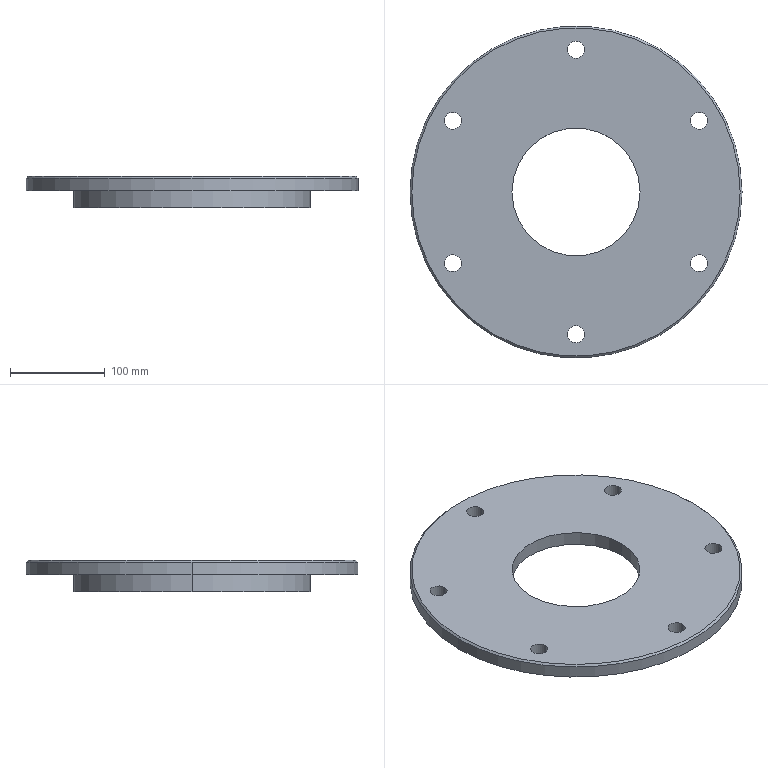Part | SolidWorks | features ICE 2, Chamfer 1, Extrusion 1 | 1 solid | 26 faces | box 350 x 350 x 33 mm | volume 1402702 mm3 | cylinder 20 | plane 4 | cone 2 | commonest cylinder face diameters 18 x12 135 x2 220 x2 250 x2 350 x2
STEP:
#1=CARTESIAN_POINT('',(-67.5,0.,18.));
#2=VERTEX_POINT('',#1);
#3=CARTESIAN_POINT('',(67.5,0.,18.));
#4=VERTEX_POINT('',#3);
#5=CARTESIAN_POINT('',(0.,0.,18.));
#6=DIRECTION('',(0.,0.,1.));
#7=DIRECTION('',(1.,0.,0.));
#8=AXIS2_PLACEMENT_3D('',#5,#6,#7);
#9=CIRCLE('',#8,67.5);
#10=EDGE_CURVE('',#2,#4,#9,.T.);
#11=ORIENTED_EDGE('',*,*,#10,.F.);
#12=CARTESIAN_POINT('',(-67.5,0.,33.));
#13=VERTEX_POINT('',#12);
#14=CARTESIAN_POINT('',(-67.5,0.,0.));
#15=DIRECTION('',(0.,0.,1.));
#16=VECTOR('',#15,1000.);
#17=LINE('',#14,#16);
#18=EDGE_CURVE('',#2,#13,#17,.T.);
#19=ORIENTED_EDGE('',*,*,#18,.T.);
#20=CARTESIAN_POINT('',(67.5,0.,33.));
#21=VERTEX_POINT('',#20);
#22=CARTESIAN_POINT('',(0.,0.,33.));
#23=DIRECTION('',(0.,0.,1.));
#24=DIRECTION('',(1.,0.,0.));
#25=AXIS2_PLACEMENT_3D('',#22,#23,#24);
#26=CIRCLE('',#25,67.5);
#27=EDGE_CURVE('',#13,#21,#26,.T.);
#28=ORIENTED_EDGE('',*,*,#27,.T.);
#29=CARTESIAN_POINT('',(67.5,0.,0.));
#30=DIRECTION('',(0.,0.,1.));
#31=VECTOR('',#30,1000.);
#32=LINE('',#29,#31);
#33=EDGE_CURVE('',#4,#21,#32,.T.);
#34=ORIENTED_EDGE('',*,*,#33,.F.);
#35=EDGE_LOOP('',(#11,#19,#28,#34));
#36=FACE_OUTER_BOUND('',#35,.T.);
#37=CARTESIAN_POINT('',(0.,0.,0.));
#38=DIRECTION('',(0.,0.,1.));
#39=DIRECTION('',(1.,0.,0.));
#40=AXIS2_PLACEMENT_3D('',#37,#38,#39);
#41=CYLINDRICAL_SURFACE('',#40,67.5);
#42=ADVANCED_FACE('',(#36),#41,.F.);
#43=CARTESIAN_POINT('',(173.,0.,33.));
#44=VERTEX_POINT('',#43);
#45=CARTESIAN_POINT('',(-173.,0.,33.));
#46=VERTEX_POINT('',#45);
#47=CARTESIAN_POINT('',(0.,0.,33.));
#48=DIRECTION('',(0.,0.,1.));
#49=DIRECTION('',(1.,0.,0.));
#50=AXIS2_PLACEMENT_3D('',#47,#48,#49);
#51=CIRCLE('',#50,173.);
#52=EDGE_CURVE('',#44,#46,#51,.T.);
#53=ORIENTED_EDGE('',*,*,#52,.F.);
#54=CARTESIAN_POINT('',(175.,0.,31.));
#55=VERTEX_POINT('',#54);
#56=CARTESIAN_POINT('',(173.,0.,33.));
#57=DIRECTION('',(0.7071,0.,-0.7071));
#58=VECTOR('',#57,1000.);
#59=LINE('',#56,#58);
#60=EDGE_CURVE('',#44,#55,#59,.T.);
#61=ORIENTED_EDGE('',*,*,#60,.T.);
#62=CARTESIAN_POINT('',(-175.,0.,31.));
#63=VERTEX_POINT('',#62);
#64=CARTESIAN_POINT('',(0.,0.,31.));
#65=DIRECTION('',(0.,0.,-1.));
#66=DIRECTION('',(1.,0.,0.));
#67=AXIS2_PLACEMENT_3D('',#64,#65,#66);
#68=CIRCLE('',#67,175.);
#69=EDGE_CURVE('',#63,#55,#68,.T.);
#70=ORIENTED_EDGE('',*,*,#69,.F.);
#71=CARTESIAN_POINT('',(-173.,0.,33.));
#72=DIRECTION('',(-0.7071,0.,-0.7071));
#73=VECTOR('',#72,1000.);
#74=LINE('',#71,#73);
#75=EDGE_CURVE('',#46,#63,#74,.T.);
#76=ORIENTED_EDGE('',*,*,#75,.F.);
#77=EDGE_LOOP('',(#53,#61,#70,#76));
#78=FACE_OUTER_BOUND('',#77,.T.);
#79=CARTESIAN_POINT('',(0.,0.,33.));
#80=DIRECTION('',(0.,0.,-1.));
#81=DIRECTION('',(-1.,0.,0.));
#82=AXIS2_PLACEMENT_3D('',#79,#80,#81);
#83=CONICAL_SURFACE('',#82,173.,0.7854);
#84=ADVANCED_FACE('',(#78),#83,.T.);
#85=CARTESIAN_POINT('',(120.904,75.,33.));
#86=VERTEX_POINT('',#85);
#87=CARTESIAN_POINT('',(138.904,75.,33.));
#88=VERTEX_POINT('',#87);
#89=CARTESIAN_POINT('',(129.904,75.,33.));
#90=DIRECTION('',(0.,0.,1.));
#91=DIRECTION('',(1.,0.,0.));
#92=AXIS2_PLACEMENT_3D('',#89,#90,#91);
#93=CIRCLE('',#92,9.);
#94=EDGE_CURVE('',#86,#88,#93,.T.);
#95=ORIENTED_EDGE('',*,*,#94,.T.);
#96=CARTESIAN_POINT('',(138.904,75.,18.));
#97=VERTEX_POINT('',#96);
#98=CARTESIAN_POINT('',(138.904,75.,33.));
#99=DIRECTION('',(0.,0.,-1.));
#100=VECTOR('',#99,1000.);
#101=LINE('',#98,#100);
#102=EDGE_CURVE('',#88,#97,#101,.T.);
#103=ORIENTED_EDGE('',*,*,#102,.T.);
#104=CARTESIAN_POINT('',(120.904,75.,18.));
#105=VERTEX_POINT('',#104);
#106=CARTESIAN_POINT('',(129.904,75.,18.));
#107=DIRECTION('',(0.,0.,1.));
#108=DIRECTION('',(1.,0.,0.));
#109=AXIS2_PLACEMENT_3D('',#106,#107,#108);
#110=CIRCLE('',#109,9.);
#111=EDGE_CURVE('',#105,#97,#110,.T.);
#112=ORIENTED_EDGE('',*,*,#111,.F.);
#113=CARTESIAN_POINT('',(120.904,75.,33.));
#114=DIRECTION('',(0.,0.,-1.));
#115=VECTOR('',#114,1000.);
#116=LINE('',#113,#115);
#117=EDGE_CURVE('',#86,#105,#116,.T.);
#118=ORIENTED_EDGE('',*,*,#117,.F.);
#119=EDGE_LOOP('',(#95,#103,#112,#118));
#120=FACE_OUTER_BOUND('',#119,.T.);
#121=CARTESIAN_POINT('',(129.904,75.,33.));
#122=DIRECTION('',(0.,0.,-1.));
#123=DIRECTION('',(-1.,0.,0.));
#124=AXIS2_PLACEMENT_3D('',#121,#122,#123);
#125=CYLINDRICAL_SURFACE('',#124,9.);
#126=ADVANCED_FACE('',(#120),#125,.F.);
#127=CARTESIAN_POINT('',(120.904,-75.,33.));
#128=VERTEX_POINT('',#127);
#129=CARTESIAN_POINT('',(138.904,-75.,33.));
#130=VERTEX_POINT('',#129);
#131=CARTESIAN_POINT('',(129.904,-75.,33.));
#132=DIRECTION('',(0.,0.,1.));
#133=DIRECTION('',(1.,0.,0.));
#134=AXIS2_PLACEMENT_3D('',#131,#132,#133);
#135=CIRCLE('',#134,9.);
#136=EDGE_CURVE('',#128,#130,#135,.T.);
#137=ORIENTED_EDGE('',*,*,#136,.T.);
#138=CARTESIAN_POINT('',(138.904,-75.,18.));
#139=VERTEX_POINT('',#138);
#140=CARTESIAN_POINT('',(138.904,-75.,33.));
#141=DIRECTION('',(0.,0.,-1.));
#142=VECTOR('',#141,1000.);
#143=LINE('',#140,#142);
#144=EDGE_CURVE('',#130,#139,#143,.T.);
#145=ORIENTED_EDGE('',*,*,#144,.T.);
#146=CARTESIAN_POINT('',(120.904,-75.,18.));
#147=VERTEX_POINT('',#146);
#148=CARTESIAN_POINT('',(129.904,-75.,18.));
#149=DIRECTION('',(0.,0.,1.));
#150=DIRECTION('',(1.,0.,0.));
#151=AXIS2_PLACEMENT_3D('',#148,#149,#150);
#152=CIRCLE('',#151,9.);
#153=EDGE_CURVE('',#147,#139,#152,.T.);
#154=ORIENTED_EDGE('',*,*,#153,.F.);
#155=CARTESIAN_POINT('',(120.904,-75.,33.));
#156=DIRECTION('',(0.,0.,-1.));
#157=VECTOR('',#156,1000.);
#158=LINE('',#155,#157);
#159=EDGE_CURVE('',#128,#147,#158,.T.);
#160=ORIENTED_EDGE('',*,*,#159,.F.);
#161=EDGE_LOOP('',(#137,#145,#154,#160));
#162=FACE_OUTER_BOUND('',#161,.T.);
#163=CARTESIAN_POINT('',(129.904,-75.,33.));
#164=DIRECTION('',(0.,0.,-1.));
#165=DIRECTION('',(-1.,0.,0.));
#166=AXIS2_PLACEMENT_3D('',#163,#164,#165);
#167=CYLINDRICAL_SURFACE('',#166,9.);
#168=ADVANCED_FACE('',(#162),#167,.F.);
#169=CARTESIAN_POINT('',(-9.,-150.,33.));
#170=VERTEX_POINT('',#169);
#171=CARTESIAN_POINT('',(9.,-150.,33.));
#172=VERTEX_POINT('',#171);
#173=CARTESIAN_POINT('',(0.,-150.,33.));
#174=DIRECTION('',(0.,0.,1.));
#175=DIRECTION('',(1.,0.,0.));
#176=AXIS2_PLACEMENT_3D('',#173,#174,#175);
#177=CIRCLE('',#176,9.);
#178=EDGE_CURVE('',#170,#172,#177,.T.);
#179=ORIENTED_EDGE('',*,*,#178,.T.);
#180=CARTESIAN_POINT('',(9.,-150.,18.));
#181=VERTEX_POINT('',#180);
#182=CARTESIAN_POINT('',(9.,-150.,33.));
#183=DIRECTION('',(0.,0.,-1.));
#184=VECTOR('',#183,1000.);
#185=LINE('',#182,#184);
#186=EDGE_CURVE('',#172,#181,#185,.T.);
#187=ORIENTED_EDGE('',*,*,#186,.T.);
#188=CARTESIAN_POINT('',(-9.,-150.,18.));
#189=VERTEX_POINT('',#188);
#190=CARTESIAN_POINT('',(0.,-150.,18.));
#191=DIRECTION('',(0.,0.,1.));
#192=DIRECTION('',(1.,0.,0.));
#193=AXIS2_PLACEMENT_3D('',#190,#191,#192);
#194=CIRCLE('',#193,9.);
#195=EDGE_CURVE('',#189,#181,#194,.T.);
#196=ORIENTED_EDGE('',*,*,#195,.F.);
#197=CARTESIAN_POINT('',(-9.,-150.,33.));
#198=DIRECTION('',(0.,0.,-1.));
#199=VECTOR('',#198,1000.);
#200=LINE('',#197,#199);
#201=EDGE_CURVE('',#170,#189,#200,.T.);
#202=ORIENTED_EDGE('',*,*,#201,.F.);
#203=EDGE_LOOP('',(#179,#187,#196,#202));
#204=FACE_OUTER_BOUND('',#203,.T.);
#205=CARTESIAN_POINT('',(0.,-150.,33.));
#206=DIRECTION('',(0.,0.,-1.));
#207=DIRECTION('',(-1.,0.,0.));
#208=AXIS2_PLACEMENT_3D('',#205,#206,#207);
#209=CYLINDRICAL_SURFACE('',#208,9.);
#210=ADVANCED_FACE('',(#204),#209,.F.);
#211=CARTESIAN_POINT('',(-138.904,-75.,33.));
#212=VERTEX_POINT('',#211);
#213=CARTESIAN_POINT('',(-120.904,-75.,33.));
#214=VERTEX_POINT('',#213);
#215=CARTESIAN_POINT('',(-129.904,-75.,33.));
#216=DIRECTION('',(0.,0.,1.));
#217=DIRECTION('',(1.,0.,0.));
#218=AXIS2_PLACEMENT_3D('',#215,#216,#217);
#219=CIRCLE('',#218,9.);
#220=EDGE_CURVE('',#212,#214,#219,.T.);
#221=ORIENTED_EDGE('',*,*,#220,.T.);
#222=CARTESIAN_POINT('',(-120.904,-75.,18.));
#223=VERTEX_POINT('',#222);
#224=CARTESIAN_POINT('',(-120.904,-75.,33.));
#225=DIRECTION('',(0.,0.,-1.));
#226=VECTOR('',#225,1000.);
#227=LINE('',#224,#226);
#228=EDGE_CURVE('',#214,#223,#227,.T.);
#229=ORIENTED_EDGE('',*,*,#228,.T.);
#230=CARTESIAN_POINT('',(-138.904,-75.,18.));
#231=VERTEX_POINT('',#230);
#232=CARTESIAN_POINT('',(-129.904,-75.,18.));
#233=DIRECTION('',(0.,0.,1.));
#234=DIRECTION('',(1.,0.,0.));
#235=AXIS2_PLACEMENT_3D('',#232,#233,#234);
#236=CIRCLE('',#235,9.);
#237=EDGE_CURVE('',#231,#223,#236,.T.);
#238=ORIENTED_EDGE('',*,*,#237,.F.);
#239=CARTESIAN_POINT('',(-138.904,-75.,33.));
#240=DIRECTION('',(0.,0.,-1.));
#241=VECTOR('',#240,1000.);
#242=LINE('',#239,#241);
#243=EDGE_CURVE('',#212,#231,#242,.T.);
#244=ORIENTED_EDGE('',*,*,#243,.F.);
#245=EDGE_LOOP('',(#221,#229,#238,#244));
#246=FACE_OUTER_BOUND('',#245,.T.);
#247=CARTESIAN_POINT('',(-129.904,-75.,33.));
#248=DIRECTION('',(0.,0.,-1.));
#249=DIRECTION('',(-1.,0.,0.));
#250=AXIS2_PLACEMENT_3D('',#247,#248,#249);
#251=CYLINDRICAL_SURFACE('',#250,9.);
#252=ADVANCED_FACE('',(#246),#251,.F.);
#253=CARTESIAN_POINT('',(-138.904,75.,33.));
#254=VERTEX_POINT('',#253);
#255=CARTESIAN_POINT('',(-120.904,75.,33.));
#256=VERTEX_POINT('',#255);
#257=CARTESIAN_POINT('',(-129.904,75.,33.));
#258=DIRECTION('',(0.,0.,1.));
#259=DIRECTION('',(1.,0.,0.));
#260=AXIS2_PLACEMENT_3D('',#257,#258,#259);
#261=CIRCLE('',#260,9.);
#262=EDGE_CURVE('',#254,#256,#261,.T.);
#263=ORIENTED_EDGE('',*,*,#262,.T.);
#264=CARTESIAN_POINT('',(-120.904,75.,18.));
#265=VERTEX_POINT('',#264);
#266=CARTESIAN_POINT('',(-120.904,75.,33.));
#267=DIRECTION('',(0.,0.,-1.));
#268=VECTOR('',#267,1000.);
#269=LINE('',#266,#268);
#270=EDGE_CURVE('',#256,#265,#269,.T.);
#271=ORIENTED_EDGE('',*,*,#270,.T.);
#272=CARTESIAN_POINT('',(-138.904,75.,18.));
#273=VERTEX_POINT('',#272);
#274=CARTESIAN_POINT('',(-129.904,75.,18.));
#275=DIRECTION('',(0.,0.,1.));
#276=DIRECTION('',(1.,0.,0.));
#277=AXIS2_PLACEMENT_3D('',#274,#275,#276);
#278=CIRCLE('',#277,9.);
#279=EDGE_CURVE('',#273,#265,#278,.T.);
#280=ORIENTED_EDGE('',*,*,#279,.F.);
#281=CARTESIAN_POINT('',(-138.904,75.,33.));
#282=DIRECTION('',(0.,0.,-1.));
#283=VECTOR('',#282,1000.);
#284=LINE('',#281,#283);
#285=EDGE_CURVE('',#254,#273,#284,.T.);
#286=ORIENTED_EDGE('',*,*,#285,.F.);
#287=EDGE_LOOP('',(#263,#271,#280,#286));
#288=FACE_OUTER_BOUND('',#287,.T.);
#289=CARTESIAN_POINT('',(-129.904,75.,33.));
#290=DIRECTION('',(0.,0.,-1.));
#291=DIRECTION('',(-1.,0.,0.));
#292=AXIS2_PLACEMENT_3D('',#289,#290,#291);
#293=CYLINDRICAL_SURFACE('',#292,9.);
#294=ADVANCED_FACE('',(#288),#293,.F.);
#295=CARTESIAN_POINT('',(-9.,150.,33.));
#296=VERTEX_POINT('',#295);
#297=CARTESIAN_POINT('',(9.,150.,33.));
#298=VERTEX_POINT('',#297);
#299=CARTESIAN_POINT('',(0.,150.,33.));
#300=DIRECTION('',(0.,0.,1.));
#301=DIRECTION('',(1.,0.,0.));
#302=AXIS2_PLACEMENT_3D('',#299,#300,#301);
#303=CIRCLE('',#302,9.);
#304=EDGE_CURVE('',#296,#298,#303,.T.);
#305=ORIENTED_EDGE('',*,*,#304,.T.);
#306=CARTESIAN_POINT('',(9.,150.,18.));
#307=VERTEX_POINT('',#306);
#308=CARTESIAN_POINT('',(9.,150.,33.));
#309=DIRECTION('',(0.,0.,-1.));
#310=VECTOR('',#309,1000.);
#311=LINE('',#308,#310);
#312=EDGE_CURVE('',#298,#307,#311,.T.);
#313=ORIENTED_EDGE('',*,*,#312,.T.);
#314=CARTESIAN_POINT('',(-9.,150.,18.));
#315=VERTEX_POINT('',#314);
#316=CARTESIAN_POINT('',(0.,150.,18.));
#317=DIRECTION('',(0.,0.,1.));
#318=DIRECTION('',(1.,0.,0.));
#319=AXIS2_PLACEMENT_3D('',#316,#317,#318);
#320=CIRCLE('',#319,9.);
#321=EDGE_CURVE('',#315,#307,#320,.T.);
#322=ORIENTED_EDGE('',*,*,#321,.F.);
#323=CARTESIAN_POINT('',(-9.,150.,33.));
#324=DIRECTION('',(0.,0.,-1.));
#325=VECTOR('',#324,1000.);
#326=LINE('',#323,#325);
#327=EDGE_CURVE('',#296,#315,#326,.T.);
#328=ORIENTED_EDGE('',*,*,#327,.F.);
#329=EDGE_LOOP('',(#305,#313,#322,#328));
#330=FACE_OUTER_BOUND('',#329,.T.);
#331=CARTESIAN_POINT('',(0.,150.,33.));
#332=DIRECTION('',(0.,0.,-1.));
#333=DIRECTION('',(-1.,0.,0.));
#334=AXIS2_PLACEMENT_3D('',#331,#332,#333);
#335=CYLINDRICAL_SURFACE('',#334,9.);
#336=ADVANCED_FACE('',(#330),#335,.F.);
#337=ORIENTED_EDGE('',*,*,#69,.T.);
#338=CARTESIAN_POINT('',(175.,0.,18.));
#339=VERTEX_POINT('',#338);
#340=CARTESIAN_POINT('',(175.,0.,33.));
#341=DIRECTION('',(0.,0.,-1.));
#342=VECTOR('',#341,1000.);
#343=LINE('',#340,#342);
#344=EDGE_CURVE('',#55,#339,#343,.T.);
#345=ORIENTED_EDGE('',*,*,#344,.T.);
#346=CARTESIAN_POINT('',(-175.,0.,18.));
#347=VERTEX_POINT('',#346);
#348=CARTESIAN_POINT('',(0.,0.,18.));
#349=DIRECTION('',(0.,0.,1.));
#350=DIRECTION('',(1.,0.,0.));
#351=AXIS2_PLACEMENT_3D('',#348,#349,#350);
#352=CIRCLE('',#351,175.);
#353=EDGE_CURVE('',#339,#347,#352,.T.);
#354=ORIENTED_EDGE('',*,*,#353,.T.);
#355=CARTESIAN_POINT('',(-175.,0.,33.));
#356=DIRECTION('',(0.,0.,-1.));
#357=VECTOR('',#356,1000.);
#358=LINE('',#355,#357);
#359=EDGE_CURVE('',#63,#347,#358,.T.);
#360=ORIENTED_EDGE('',*,*,#359,.F.);
#361=EDGE_LOOP('',(#337,#345,#354,#360));
#362=FACE_OUTER_BOUND('',#361,.T.);
#363=CARTESIAN_POINT('',(0.,0.,33.));
#364=DIRECTION('',(0.,0.,-1.));
#365=DIRECTION('',(-1.,0.,0.));
#366=AXIS2_PLACEMENT_3D('',#363,#364,#365);
#367=CYLINDRICAL_SURFACE('',#366,175.);
#368=ADVANCED_FACE('',(#362),#367,.T.);
#369=CARTESIAN_POINT('',(110.,0.,18.));
#370=VERTEX_POINT('',#369);
#371=CARTESIAN_POINT('',(-110.,0.,18.));
#372=VERTEX_POINT('',#371);
#373=CARTESIAN_POINT('',(0.,0.,18.));
#374=DIRECTION('',(0.,0.,-1.));
#375=DIRECTION('',(-1.,0.,0.));
#376=AXIS2_PLACEMENT_3D('',#373,#374,#375);
#377=CIRCLE('',#376,110.);
#378=EDGE_CURVE('',#370,#372,#377,.T.);
#379=ORIENTED_EDGE('',*,*,#378,.F.);
#380=CARTESIAN_POINT('',(110.,0.,0.));
#381=VERTEX_POINT('',#380);
#382=CARTESIAN_POINT('',(110.,0.,371.553));
#383=DIRECTION('',(0.,0.,-1.));
#384=VECTOR('',#383,1000.);
#385=LINE('',#382,#384);
#386=EDGE_CURVE('',#370,#381,#385,.T.);
#387=ORIENTED_EDGE('',*,*,#386,.T.);
#388=CARTESIAN_POINT('',(-110.,0.,0.));
#389=VERTEX_POINT('',#388);
#390=CARTESIAN_POINT('',(0.,0.,0.));
#391=DIRECTION('',(0.,0.,1.));
#392=DIRECTION('',(1.,0.,0.));
#393=AXIS2_PLACEMENT_3D('',#390,#391,#392);
#394=CIRCLE('',#393,110.);
#395=EDGE_CURVE('',#389,#381,#394,.T.);
#396=ORIENTED_EDGE('',*,*,#395,.F.);
#397=CARTESIAN_POINT('',(-110.,0.,371.553));
#398=DIRECTION('',(0.,0.,-1.));
#399=VECTOR('',#398,1000.);
#400=LINE('',#397,#399);
#401=EDGE_CURVE('',#372,#389,#400,.T.);
#402=ORIENTED_EDGE('',*,*,#401,.F.);
#403=EDGE_LOOP('',(#379,#387,#396,#402));
#404=FACE_OUTER_BOUND('',#403,.T.);
#405=CARTESIAN_POINT('',(0.,0.,371.553));
#406=DIRECTION('',(0.,0.,-1.));
#407=DIRECTION('',(-1.,0.,0.));
#408=AXIS2_PLACEMENT_3D('',#405,#406,#407);
#409=CYLINDRICAL_SURFACE('',#408,110.);
#410=ADVANCED_FACE('',(#404),#409,.F.);
#411=CARTESIAN_POINT('',(125.,0.,18.));
#412=VERTEX_POINT('',#411);
#413=CARTESIAN_POINT('',(-125.,0.,18.));
#414=VERTEX_POINT('',#413);
#415=CARTESIAN_POINT('',(0.,0.,18.));
#416=DIRECTION('',(0.,0.,1.));
#417=DIRECTION('',(1.,0.,0.));
#418=AXIS2_PLACEMENT_3D('',#415,#416,#417);
#419=CIRCLE('',#418,125.);
#420=EDGE_CURVE('',#412,#414,#419,.T.);
#421=ORIENTED_EDGE('',*,*,#420,.F.);
#422=CARTESIAN_POINT('',(125.,0.,0.));
#423=VERTEX_POINT('',#422);
#424=CARTESIAN_POINT('',(125.,0.,371.553));
#425=DIRECTION('',(0.,0.,-1.));
#426=VECTOR('',#425,1000.);
#427=LINE('',#424,#426);
#428=EDGE_CURVE('',#412,#423,#427,.T.);
#429=ORIENTED_EDGE('',*,*,#428,.T.);
#430=CARTESIAN_POINT('',(-125.,0.,0.));
#431=VERTEX_POINT('',#430);
#432=CARTESIAN_POINT('',(0.,0.,0.));
#433=DIRECTION('',(0.,0.,1.));
#434=DIRECTION('',(1.,0.,0.));
#435=AXIS2_PLACEMENT_3D('',#432,#433,#434);
#436=CIRCLE('',#435,125.);
#437=EDGE_CURVE('',#423,#431,#436,.T.);
#438=ORIENTED_EDGE('',*,*,#437,.T.);
#439=CARTESIAN_POINT('',(-125.,0.,371.553));
#440=DIRECTION('',(0.,0.,-1.));
#441=VECTOR('',#440,1000.);
#442=LINE('',#439,#441);
#443=EDGE_CURVE('',#414,#431,#442,.T.);
#444=ORIENTED_EDGE('',*,*,#443,.F.);
#445=EDGE_LOOP('',(#421,#429,#438,#444));
#446=FACE_OUTER_BOUND('',#445,.T.);
#447=CARTESIAN_POINT('',(0.,0.,371.553));
#448=DIRECTION('',(0.,0.,-1.));
#449=DIRECTION('',(-1.,0.,0.));
#450=AXIS2_PLACEMENT_3D('',#447,#448,#449);
#451=CYLINDRICAL_SURFACE('',#450,125.);
#452=ADVANCED_FACE('',(#446),#451,.T.);
#453=CARTESIAN_POINT('',(0.,0.,0.));
#454=DIRECTION('',(0.,0.,1.));
#455=DIRECTION('',(1.,0.,0.));
#456=AXIS2_PLACEMENT_3D('',#453,#454,#455);
#457=CIRCLE('',#456,125.);
#458=EDGE_CURVE('',#431,#423,#457,.T.);
#459=ORIENTED_EDGE('',*,*,#458,.F.);
#460=ORIENTED_EDGE('',*,*,#437,.F.);
#461=EDGE_LOOP('',(#459,#460));
#462=FACE_OUTER_BOUND('',#461,.T.);
#463=ORIENTED_EDGE('',*,*,#395,.T.);
#464=CARTESIAN_POINT('',(0.,0.,0.));
#465=DIRECTION('',(0.,0.,1.));
#466=DIRECTION('',(1.,0.,0.));
#467=AXIS2_PLACEMENT_3D('',#464,#465,#466);
#468=CIRCLE('',#467,110.);
#469=EDGE_CURVE('',#381,#389,#468,.T.);
#470=ORIENTED_EDGE('',*,*,#469,.T.);
#471=EDGE_LOOP('',(#463,#470));
#472=FACE_BOUND('',#471,.T.);
#473=CARTESIAN_POINT('',(0.,0.,0.));
#474=DIRECTION('',(0.,0.,1.));
#475=DIRECTION('',(1.,0.,0.));
#476=AXIS2_PLACEMENT_3D('',#473,#474,#475);
#477=PLANE('',#476);
#478=ADVANCED_FACE('',(#462,#472),#477,.F.);
#479=ORIENTED_EDGE('',*,*,#428,.F.);
#480=CARTESIAN_POINT('',(0.,0.,18.));
#481=DIRECTION('',(0.,0.,1.));
#482=DIRECTION('',(1.,0.,0.));
#483=AXIS2_PLACEMENT_3D('',#480,#481,#482);
#484=CIRCLE('',#483,125.);
#485=EDGE_CURVE('',#414,#412,#484,.T.);
#486=ORIENTED_EDGE('',*,*,#485,.F.);
#487=ORIENTED_EDGE('',*,*,#443,.T.);
#488=ORIENTED_EDGE('',*,*,#458,.T.);
#489=EDGE_LOOP('',(#479,#486,#487,#488));
#490=FACE_OUTER_BOUND('',#489,.T.);
#491=CARTESIAN_POINT('',(0.,0.,371.553));
#492=DIRECTION('',(0.,0.,-1.));
#493=DIRECTION('',(-1.,0.,0.));
#494=AXIS2_PLACEMENT_3D('',#491,#492,#493);
#495=CYLINDRICAL_SURFACE('',#494,125.);
#496=ADVANCED_FACE('',(#490),#495,.T.);
#497=ORIENTED_EDGE('',*,*,#386,.F.);
#498=CARTESIAN_POINT('',(0.,0.,18.));
#499=DIRECTION('',(0.,0.,-1.));
#500=DIRECTION('',(-1.,0.,0.));
#501=AXIS2_PLACEMENT_3D('',#498,#499,#500);
#502=CIRCLE('',#501,110.);
#503=EDGE_CURVE('',#372,#370,#502,.T.);
#504=ORIENTED_EDGE('',*,*,#503,.F.);
#505=ORIENTED_EDGE('',*,*,#401,.T.);
#506=ORIENTED_EDGE('',*,*,#469,.F.);
#507=EDGE_LOOP('',(#497,#504,#505,#506));
#508=FACE_OUTER_BOUND('',#507,.T.);
#509=CARTESIAN_POINT('',(0.,0.,371.553));
#510=DIRECTION('',(0.,0.,-1.));
#511=DIRECTION('',(-1.,0.,0.));
#512=AXIS2_PLACEMENT_3D('',#509,#510,#511);
#513=CYLINDRICAL_SURFACE('',#512,110.);
#514=ADVANCED_FACE('',(#508),#513,.F.);
#515=CARTESIAN_POINT('',(0.,0.,18.));
#516=DIRECTION('',(0.,0.,1.));
#517=DIRECTION('',(1.,0.,0.));
#518=AXIS2_PLACEMENT_3D('',#515,#516,#517);
#519=CIRCLE('',#518,67.5);
#520=EDGE_CURVE('',#4,#2,#519,.T.);
#521=ORIENTED_EDGE('',*,*,#520,.T.);
#522=ORIENTED_EDGE('',*,*,#10,.T.);
#523=EDGE_LOOP('',(#521,#522));
#524=FACE_BOUND('',#523,.T.);
#525=ORIENTED_EDGE('',*,*,#503,.T.);
#526=ORIENTED_EDGE('',*,*,#378,.T.);
#527=EDGE_LOOP('',(#525,#526));
#528=FACE_OUTER_BOUND('',#527,.T.);
#529=CARTESIAN_POINT('',(0.,0.,18.));
#530=DIRECTION('',(0.,0.,1.));
#531=DIRECTION('',(1.,0.,0.));
#532=AXIS2_PLACEMENT_3D('',#529,#530,#531);
#533=PLANE('',#532);
#534=ADVANCED_FACE('',(#524,#528),#533,.F.);
#535=ORIENTED_EDGE('',*,*,#153,.T.);
#536=CARTESIAN_POINT('',(129.904,-75.,18.));
#537=DIRECTION('',(0.,0.,1.));
#538=DIRECTION('',(1.,0.,0.));
#539=AXIS2_PLACEMENT_3D('',#536,#537,#538);
#540=CIRCLE('',#539,9.);
#541=EDGE_CURVE('',#139,#147,#540,.T.);
#542=ORIENTED_EDGE('',*,*,#541,.T.);
#543=EDGE_LOOP('',(#535,#542));
#544=FACE_BOUND('',#543,.T.);
#545=ORIENTED_EDGE('',*,*,#237,.T.);
#546=CARTESIAN_POINT('',(-129.904,-75.,18.));
#547=DIRECTION('',(0.,0.,1.));
#548=DIRECTION('',(1.,0.,0.));
#549=AXIS2_PLACEMENT_3D('',#546,#547,#548);
#550=CIRCLE('',#549,9.);
#551=EDGE_CURVE('',#223,#231,#550,.T.);
#552=ORIENTED_EDGE('',*,*,#551,.T.);
#553=EDGE_LOOP('',(#545,#552));
#554=FACE_BOUND('',#553,.T.);
#555=ORIENTED_EDGE('',*,*,#321,.T.);
#556=CARTESIAN_POINT('',(0.,150.,18.));
#557=DIRECTION('',(0.,0.,1.));
#558=DIRECTION('',(1.,0.,0.));
#559=AXIS2_PLACEMENT_3D('',#556,#557,#558);
#560=CIRCLE('',#559,9.);
#561=EDGE_CURVE('',#307,#315,#560,.T.);
#562=ORIENTED_EDGE('',*,*,#561,.T.);
#563=EDGE_LOOP('',(#555,#562));
#564=FACE_BOUND('',#563,.T.);
#565=CARTESIAN_POINT('',(0.,0.,18.));
#566=DIRECTION('',(0.,0.,1.));
#567=DIRECTION('',(1.,0.,0.));
#568=AXIS2_PLACEMENT_3D('',#565,#566,#567);
#569=CIRCLE('',#568,175.);
#570=EDGE_CURVE('',#347,#339,#569,.T.);
#571=ORIENTED_EDGE('',*,*,#570,.F.);
#572=ORIENTED_EDGE('',*,*,#353,.F.);
#573=EDGE_LOOP('',(#571,#572));
#574=FACE_OUTER_BOUND('',#573,.T.);
#575=ORIENTED_EDGE('',*,*,#279,.T.);
#576=CARTESIAN_POINT('',(-129.904,75.,18.));
#577=DIRECTION('',(0.,0.,1.));
#578=DIRECTION('',(1.,0.,0.));
#579=AXIS2_PLACEMENT_3D('',#576,#577,#578);
#580=CIRCLE('',#579,9.);
#581=EDGE_CURVE('',#265,#273,#580,.T.);
#582=ORIENTED_EDGE('',*,*,#581,.T.);
#583=EDGE_LOOP('',(#575,#582));
#584=FACE_BOUND('',#583,.T.);
#585=ORIENTED_EDGE('',*,*,#195,.T.);
#586=CARTESIAN_POINT('',(0.,-150.,18.));
#587=DIRECTION('',(0.,0.,1.));
#588=DIRECTION('',(1.,0.,0.));
#589=AXIS2_PLACEMENT_3D('',#586,#587,#588);
#590=CIRCLE('',#589,9.);
#591=EDGE_CURVE('',#181,#189,#590,.T.);
#592=ORIENTED_EDGE('',*,*,#591,.T.);
#593=EDGE_LOOP('',(#585,#592));
#594=FACE_BOUND('',#593,.T.);
#595=ORIENTED_EDGE('',*,*,#111,.T.);
#596=CARTESIAN_POINT('',(129.904,75.,18.));
#597=DIRECTION('',(0.,0.,1.));
#598=DIRECTION('',(1.,0.,0.));
#599=AXIS2_PLACEMENT_3D('',#596,#597,#598);
#600=CIRCLE('',#599,9.);
#601=EDGE_CURVE('',#97,#105,#600,.T.);
#602=ORIENTED_EDGE('',*,*,#601,.T.);
#603=EDGE_LOOP('',(#595,#602));
#604=FACE_BOUND('',#603,.T.);
#605=ORIENTED_EDGE('',*,*,#485,.T.);
#606=ORIENTED_EDGE('',*,*,#420,.T.);
#607=EDGE_LOOP('',(#605,#606));
#608=FACE_BOUND('',#607,.T.);
#609=CARTESIAN_POINT('',(0.,0.,18.));
#610=DIRECTION('',(0.,0.,1.));
#611=DIRECTION('',(1.,0.,0.));
#612=AXIS2_PLACEMENT_3D('',#609,#610,#611);
#613=PLANE('',#612);
#614=ADVANCED_FACE('',(#544,#554,#564,#574,#584,#594,#604,#608),#613,.F.);
#615=CARTESIAN_POINT('',(0.,0.,33.));
#616=DIRECTION('',(0.,0.,1.));
#617=DIRECTION('',(1.,0.,0.));
#618=AXIS2_PLACEMENT_3D('',#615,#616,#617);
#619=CIRCLE('',#618,67.5);
#620=EDGE_CURVE('',#21,#13,#619,.T.);
#621=ORIENTED_EDGE('',*,*,#620,.F.);
#622=ORIENTED_EDGE('',*,*,#27,.F.);
#623=EDGE_LOOP('',(#621,#622));
#624=FACE_BOUND('',#623,.T.);
#625=CARTESIAN_POINT('',(0.,0.,33.));
#626=DIRECTION('',(0.,0.,1.));
#627=DIRECTION('',(1.,0.,0.));
#628=AXIS2_PLACEMENT_3D('',#625,#626,#627);
#629=CIRCLE('',#628,173.);
#630=EDGE_CURVE('',#46,#44,#629,.T.);
#631=ORIENTED_EDGE('',*,*,#630,.T.);
#632=ORIENTED_EDGE('',*,*,#52,.T.);
#633=EDGE_LOOP('',(#631,#632));
#634=FACE_OUTER_BOUND('',#633,.T.);
#635=ORIENTED_EDGE('',*,*,#136,.F.);
#636=CARTESIAN_POINT('',(129.904,-75.,33.));
#637=DIRECTION('',(0.,0.,1.));
#638=DIRECTION('',(1.,0.,0.));
#639=AXIS2_PLACEMENT_3D('',#636,#637,#638);
#640=CIRCLE('',#639,9.);
#641=EDGE_CURVE('',#130,#128,#640,.T.);
#642=ORIENTED_EDGE('',*,*,#641,.F.);
#643=EDGE_LOOP('',(#635,#642));
#644=FACE_BOUND('',#643,.T.);
#645=ORIENTED_EDGE('',*,*,#220,.F.);
#646=CARTESIAN_POINT('',(-129.904,-75.,33.));
#647=DIRECTION('',(0.,0.,1.));
#648=DIRECTION('',(1.,0.,0.));
#649=AXIS2_PLACEMENT_3D('',#646,#647,#648);
#650=CIRCLE('',#649,9.);
#651=EDGE_CURVE('',#214,#212,#650,.T.);
#652=ORIENTED_EDGE('',*,*,#651,.F.);
#653=EDGE_LOOP('',(#645,#652));
#654=FACE_BOUND('',#653,.T.);
#655=ORIENTED_EDGE('',*,*,#304,.F.);
#656=CARTESIAN_POINT('',(0.,150.,33.));
#657=DIRECTION('',(0.,0.,1.));
#658=DIRECTION('',(1.,0.,0.));
#659=AXIS2_PLACEMENT_3D('',#656,#657,#658);
#660=CIRCLE('',#659,9.);
#661=EDGE_CURVE('',#298,#296,#660,.T.);
#662=ORIENTED_EDGE('',*,*,#661,.F.);
#663=EDGE_LOOP('',(#655,#662));
#664=FACE_BOUND('',#663,.T.);
#665=ORIENTED_EDGE('',*,*,#262,.F.);
#666=CARTESIAN_POINT('',(-129.904,75.,33.));
#667=DIRECTION('',(0.,0.,1.));
#668=DIRECTION('',(1.,0.,0.));
#669=AXIS2_PLACEMENT_3D('',#666,#667,#668);
#670=CIRCLE('',#669,9.);
#671=EDGE_CURVE('',#256,#254,#670,.T.);
#672=ORIENTED_EDGE('',*,*,#671,.F.);
#673=EDGE_LOOP('',(#665,#672));
#674=FACE_BOUND('',#673,.T.);
#675=ORIENTED_EDGE('',*,*,#178,.F.);
#676=CARTESIAN_POINT('',(0.,-150.,33.));
#677=DIRECTION('',(0.,0.,1.));
#678=DIRECTION('',(1.,0.,0.));
#679=AXIS2_PLACEMENT_3D('',#676,#677,#678);
#680=CIRCLE('',#679,9.);
#681=EDGE_CURVE('',#172,#170,#680,.T.);
#682=ORIENTED_EDGE('',*,*,#681,.F.);
#683=EDGE_LOOP('',(#675,#682));
#684=FACE_BOUND('',#683,.T.);
#685=ORIENTED_EDGE('',*,*,#94,.F.);
#686=CARTESIAN_POINT('',(129.904,75.,33.));
#687=DIRECTION('',(0.,0.,1.));
#688=DIRECTION('',(1.,0.,0.));
#689=AXIS2_PLACEMENT_3D('',#686,#687,#688);
#690=CIRCLE('',#689,9.);
#691=EDGE_CURVE('',#88,#86,#690,.T.);
#692=ORIENTED_EDGE('',*,*,#691,.F.);
#693=EDGE_LOOP('',(#685,#692));
#694=FACE_BOUND('',#693,.T.);
#695=CARTESIAN_POINT('',(0.,0.,33.));
#696=DIRECTION('',(0.,0.,1.));
#697=DIRECTION('',(1.,0.,0.));
#698=AXIS2_PLACEMENT_3D('',#695,#696,#697);
#699=PLANE('',#698);
#700=ADVANCED_FACE('',(#624,#634,#644,#654,#664,#674,#684,#694),#699,.T.);
#701=ORIENTED_EDGE('',*,*,#344,.F.);
#702=CARTESIAN_POINT('',(0.,0.,31.));
#703=DIRECTION('',(0.,0.,-1.));
#704=DIRECTION('',(1.,0.,0.));
#705=AXIS2_PLACEMENT_3D('',#702,#703,#704);
#706=CIRCLE('',#705,175.);
#707=EDGE_CURVE('',#55,#63,#706,.T.);
#708=ORIENTED_EDGE('',*,*,#707,.T.);
#709=ORIENTED_EDGE('',*,*,#359,.T.);
#710=ORIENTED_EDGE('',*,*,#570,.T.);
#711=EDGE_LOOP('',(#701,#708,#709,#710));
#712=FACE_OUTER_BOUND('',#711,.T.);
#713=CARTESIAN_POINT('',(0.,0.,33.));
#714=DIRECTION('',(0.,0.,-1.));
#715=DIRECTION('',(-1.,0.,0.));
#716=AXIS2_PLACEMENT_3D('',#713,#714,#715);
#717=CYLINDRICAL_SURFACE('',#716,175.);
#718=ADVANCED_FACE('',(#712),#717,.T.);
#719=ORIENTED_EDGE('',*,*,#312,.F.);
#720=ORIENTED_EDGE('',*,*,#661,.T.);
#721=ORIENTED_EDGE('',*,*,#327,.T.);
#722=ORIENTED_EDGE('',*,*,#561,.F.);
#723=EDGE_LOOP('',(#719,#720,#721,#722));
#724=FACE_OUTER_BOUND('',#723,.T.);
#725=CARTESIAN_POINT('',(0.,150.,33.));
#726=DIRECTION('',(0.,0.,-1.));
#727=DIRECTION('',(-1.,0.,0.));
#728=AXIS2_PLACEMENT_3D('',#725,#726,#727);
#729=CYLINDRICAL_SURFACE('',#728,9.);
#730=ADVANCED_FACE('',(#724),#729,.F.);
#731=ORIENTED_EDGE('',*,*,#270,.F.);
#732=ORIENTED_EDGE('',*,*,#671,.T.);
#733=ORIENTED_EDGE('',*,*,#285,.T.);
#734=ORIENTED_EDGE('',*,*,#581,.F.);
#735=EDGE_LOOP('',(#731,#732,#733,#734));
#736=FACE_OUTER_BOUND('',#735,.T.);
#737=CARTESIAN_POINT('',(-129.904,75.,33.));
#738=DIRECTION('',(0.,0.,-1.));
#739=DIRECTION('',(-1.,0.,0.));
#740=AXIS2_PLACEMENT_3D('',#737,#738,#739);
#741=CYLINDRICAL_SURFACE('',#740,9.);
#742=ADVANCED_FACE('',(#736),#741,.F.);
#743=ORIENTED_EDGE('',*,*,#228,.F.);
#744=ORIENTED_EDGE('',*,*,#651,.T.);
#745=ORIENTED_EDGE('',*,*,#243,.T.);
#746=ORIENTED_EDGE('',*,*,#551,.F.);
#747=EDGE_LOOP('',(#743,#744,#745,#746));
#748=FACE_OUTER_BOUND('',#747,.T.);
#749=CARTESIAN_POINT('',(-129.904,-75.,33.));
#750=DIRECTION('',(0.,0.,-1.));
#751=DIRECTION('',(-1.,0.,0.));
#752=AXIS2_PLACEMENT_3D('',#749,#750,#751);
#753=CYLINDRICAL_SURFACE('',#752,9.);
#754=ADVANCED_FACE('',(#748),#753,.F.);
#755=ORIENTED_EDGE('',*,*,#186,.F.);
#756=ORIENTED_EDGE('',*,*,#681,.T.);
#757=ORIENTED_EDGE('',*,*,#201,.T.);
#758=ORIENTED_EDGE('',*,*,#591,.F.);
#759=EDGE_LOOP('',(#755,#756,#757,#758));
#760=FACE_OUTER_BOUND('',#759,.T.);
#761=CARTESIAN_POINT('',(0.,-150.,33.));
#762=DIRECTION('',(0.,0.,-1.));
#763=DIRECTION('',(-1.,0.,0.));
#764=AXIS2_PLACEMENT_3D('',#761,#762,#763);
#765=CYLINDRICAL_SURFACE('',#764,9.);
#766=ADVANCED_FACE('',(#760),#765,.F.);
#767=ORIENTED_EDGE('',*,*,#144,.F.);
#768=ORIENTED_EDGE('',*,*,#641,.T.);
#769=ORIENTED_EDGE('',*,*,#159,.T.);
#770=ORIENTED_EDGE('',*,*,#541,.F.);
#771=EDGE_LOOP('',(#767,#768,#769,#770));
#772=FACE_OUTER_BOUND('',#771,.T.);
#773=CARTESIAN_POINT('',(129.904,-75.,33.));
#774=DIRECTION('',(0.,0.,-1.));
#775=DIRECTION('',(-1.,0.,0.));
#776=AXIS2_PLACEMENT_3D('',#773,#774,#775);
#777=CYLINDRICAL_SURFACE('',#776,9.);
#778=ADVANCED_FACE('',(#772),#777,.F.);
#779=ORIENTED_EDGE('',*,*,#102,.F.);
#780=ORIENTED_EDGE('',*,*,#691,.T.);
#781=ORIENTED_EDGE('',*,*,#117,.T.);
#782=ORIENTED_EDGE('',*,*,#601,.F.);
#783=EDGE_LOOP('',(#779,#780,#781,#782));
#784=FACE_OUTER_BOUND('',#783,.T.);
#785=CARTESIAN_POINT('',(129.904,75.,33.));
#786=DIRECTION('',(0.,0.,-1.));
#787=DIRECTION('',(-1.,0.,0.));
#788=AXIS2_PLACEMENT_3D('',#785,#786,#787);
#789=CYLINDRICAL_SURFACE('',#788,9.);
#790=ADVANCED_FACE('',(#784),#789,.F.);
#791=ORIENTED_EDGE('',*,*,#60,.F.);
#792=ORIENTED_EDGE('',*,*,#630,.F.);
#793=ORIENTED_EDGE('',*,*,#75,.T.);
#794=ORIENTED_EDGE('',*,*,#707,.F.);
#795=EDGE_LOOP('',(#791,#792,#793,#794));
#796=FACE_OUTER_BOUND('',#795,.T.);
#797=CARTESIAN_POINT('',(0.,0.,33.));
#798=DIRECTION('',(0.,0.,-1.));
#799=DIRECTION('',(-1.,0.,0.));
#800=AXIS2_PLACEMENT_3D('',#797,#798,#799);
#801=CONICAL_SURFACE('',#800,173.,0.7854);
#802=ADVANCED_FACE('',(#796),#801,.T.);
#803=ORIENTED_EDGE('',*,*,#18,.F.);
#804=ORIENTED_EDGE('',*,*,#520,.F.);
#805=ORIENTED_EDGE('',*,*,#33,.T.);
#806=ORIENTED_EDGE('',*,*,#620,.T.);
#807=EDGE_LOOP('',(#803,#804,#805,#806));
#808=FACE_OUTER_BOUND('',#807,.T.);
#809=CARTESIAN_POINT('',(0.,0.,0.));
#810=DIRECTION('',(0.,0.,1.));
#811=DIRECTION('',(1.,0.,0.));
#812=AXIS2_PLACEMENT_3D('',#809,#810,#811);
#813=CYLINDRICAL_SURFACE('',#812,67.5);
#814=ADVANCED_FACE('',(#808),#813,.F.);
#815=CLOSED_SHELL('',(#42,#84,#126,#168,#210,#252,#294,#336,#368,#410,#452,#478,#496,#514,#534,#614,#700,#718,#730,#742,#754,#766,#778,#790,#802,#814));
#816=MANIFOLD_SOLID_BREP('',#815);
#817=CARTESIAN_POINT('',(0.,0.,0.));
#818=DIRECTION('',(0.,0.,1.));
#819=DIRECTION('',(1.,0.,0.));
#820=AXIS2_PLACEMENT_3D('',#817,#818,#819);
#821=(LENGTH_UNIT()NAMED_UNIT(*)SI_UNIT(.MILLI.,.METRE.));
#822=UNCERTAINTY_MEASURE_WITH_UNIT(LENGTH_MEASURE(0.00001),#821,'','');
#823=(NAMED_UNIT(*)PLANE_ANGLE_UNIT()SI_UNIT($,.RADIAN.));
#824=(NAMED_UNIT(*)SI_UNIT($,.STERADIAN.)SOLID_ANGLE_UNIT());
#825=(GEOMETRIC_REPRESENTATION_CONTEXT(3)GLOBAL_UNCERTAINTY_ASSIGNED_CONTEXT((#822))GLOBAL_UNIT_ASSIGNED_CONTEXT((#821,#823,#824))REPRESENTATION_CONTEXT('',''));
#826=ADVANCED_BREP_SHAPE_REPRESENTATION('',(#816,#820),#825);